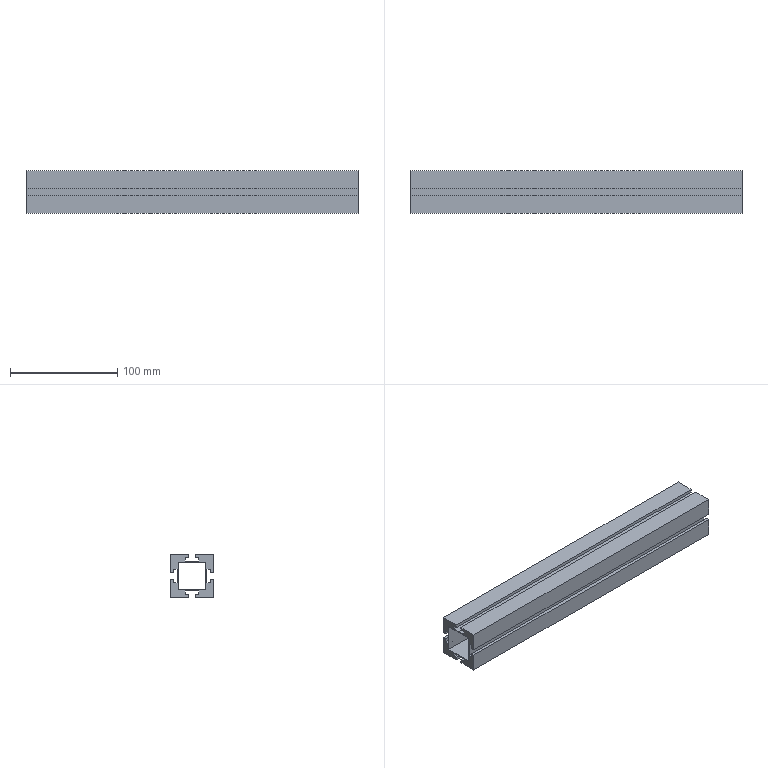Part | SolidWorks | features Extrusion 1 | 1 solid | 42 faces | box 310 x 40 x 40 mm | volume 215760 mm3 | plane 42
STEP:
#1=CARTESIAN_POINT('',(310.,3.,-20.));
#2=VERTEX_POINT('',#1);
#3=CARTESIAN_POINT('',(310.,20.,-20.));
#4=VERTEX_POINT('',#3);
#5=CARTESIAN_POINT('',(310.,3.,-20.));
#6=DIRECTION('',(0.,1.,0.));
#7=VECTOR('',#6,1000.);
#8=LINE('',#5,#7);
#9=EDGE_CURVE('',#2,#4,#8,.T.);
#10=ORIENTED_EDGE('',*,*,#9,.T.);
#11=CARTESIAN_POINT('',(310.,20.,-3.));
#12=VERTEX_POINT('',#11);
#13=CARTESIAN_POINT('',(310.,20.,-3.));
#14=DIRECTION('',(0.,0.,1.));
#15=VECTOR('',#14,1000.);
#16=LINE('',#13,#15);
#17=EDGE_CURVE('',#4,#12,#16,.T.);
#18=ORIENTED_EDGE('',*,*,#17,.T.);
#19=CARTESIAN_POINT('',(310.,17.,-3.));
#20=VERTEX_POINT('',#19);
#21=CARTESIAN_POINT('',(310.,20.,-3.));
#22=DIRECTION('',(0.,-1.,0.));
#23=VECTOR('',#22,1000.);
#24=LINE('',#21,#23);
#25=EDGE_CURVE('',#12,#20,#24,.T.);
#26=ORIENTED_EDGE('',*,*,#25,.T.);
#27=CARTESIAN_POINT('',(310.,17.,-6.5));
#28=VERTEX_POINT('',#27);
#29=CARTESIAN_POINT('',(310.,17.,-3.));
#30=DIRECTION('',(0.,0.,-1.));
#31=VECTOR('',#30,1000.);
#32=LINE('',#29,#31);
#33=EDGE_CURVE('',#20,#28,#32,.T.);
#34=ORIENTED_EDGE('',*,*,#33,.T.);
#35=CARTESIAN_POINT('',(310.,14.,-6.5));
#36=VERTEX_POINT('',#35);
#37=CARTESIAN_POINT('',(310.,17.,-6.5));
#38=DIRECTION('',(0.,-1.,0.));
#39=VECTOR('',#38,1000.);
#40=LINE('',#37,#39);
#41=EDGE_CURVE('',#28,#36,#40,.T.);
#42=ORIENTED_EDGE('',*,*,#41,.T.);
#43=CARTESIAN_POINT('',(310.,14.,6.5));
#44=VERTEX_POINT('',#43);
#45=CARTESIAN_POINT('',(310.,14.,6.5));
#46=DIRECTION('',(0.,0.,1.));
#47=VECTOR('',#46,1000.);
#48=LINE('',#45,#47);
#49=EDGE_CURVE('',#36,#44,#48,.T.);
#50=ORIENTED_EDGE('',*,*,#49,.T.);
#51=CARTESIAN_POINT('',(310.,17.,6.5));
#52=VERTEX_POINT('',#51);
#53=CARTESIAN_POINT('',(310.,17.,6.5));
#54=DIRECTION('',(0.,1.,0.));
#55=VECTOR('',#54,1000.);
#56=LINE('',#53,#55);
#57=EDGE_CURVE('',#44,#52,#56,.T.);
#58=ORIENTED_EDGE('',*,*,#57,.T.);
#59=CARTESIAN_POINT('',(310.,17.,3.));
#60=VERTEX_POINT('',#59);
#61=CARTESIAN_POINT('',(310.,17.,6.5));
#62=DIRECTION('',(0.,0.,-1.));
#63=VECTOR('',#62,1000.);
#64=LINE('',#61,#63);
#65=EDGE_CURVE('',#52,#60,#64,.T.);
#66=ORIENTED_EDGE('',*,*,#65,.T.);
#67=CARTESIAN_POINT('',(310.,20.,3.));
#68=VERTEX_POINT('',#67);
#69=CARTESIAN_POINT('',(310.,20.,3.));
#70=DIRECTION('',(0.,1.,0.));
#71=VECTOR('',#70,1000.);
#72=LINE('',#69,#71);
#73=EDGE_CURVE('',#60,#68,#72,.T.);
#74=ORIENTED_EDGE('',*,*,#73,.T.);
#75=CARTESIAN_POINT('',(310.,20.,20.));
#76=VERTEX_POINT('',#75);
#77=CARTESIAN_POINT('',(310.,20.,20.));
#78=DIRECTION('',(0.,0.,1.));
#79=VECTOR('',#78,1000.);
#80=LINE('',#77,#79);
#81=EDGE_CURVE('',#68,#76,#80,.T.);
#82=ORIENTED_EDGE('',*,*,#81,.T.);
#83=CARTESIAN_POINT('',(310.,3.,20.));
#84=VERTEX_POINT('',#83);
#85=CARTESIAN_POINT('',(310.,3.,20.));
#86=DIRECTION('',(0.,-1.,0.));
#87=VECTOR('',#86,1000.);
#88=LINE('',#85,#87);
#89=EDGE_CURVE('',#76,#84,#88,.T.);
#90=ORIENTED_EDGE('',*,*,#89,.T.);
#91=CARTESIAN_POINT('',(310.,3.,17.));
#92=VERTEX_POINT('',#91);
#93=CARTESIAN_POINT('',(310.,3.,17.));
#94=DIRECTION('',(0.,0.,-1.));
#95=VECTOR('',#94,1000.);
#96=LINE('',#93,#95);
#97=EDGE_CURVE('',#84,#92,#96,.T.);
#98=ORIENTED_EDGE('',*,*,#97,.T.);
#99=CARTESIAN_POINT('',(310.,6.5,17.));
#100=VERTEX_POINT('',#99);
#101=CARTESIAN_POINT('',(310.,3.,17.));
#102=DIRECTION('',(0.,1.,0.));
#103=VECTOR('',#102,1000.);
#104=LINE('',#101,#103);
#105=EDGE_CURVE('',#92,#100,#104,.T.);
#106=ORIENTED_EDGE('',*,*,#105,.T.);
#107=CARTESIAN_POINT('',(310.,6.5,14.));
#108=VERTEX_POINT('',#107);
#109=CARTESIAN_POINT('',(310.,6.5,14.));
#110=DIRECTION('',(0.,0.,-1.));
#111=VECTOR('',#110,1000.);
#112=LINE('',#109,#111);
#113=EDGE_CURVE('',#100,#108,#112,.T.);
#114=ORIENTED_EDGE('',*,*,#113,.T.);
#115=CARTESIAN_POINT('',(310.,-6.5,14.));
#116=VERTEX_POINT('',#115);
#117=CARTESIAN_POINT('',(310.,-6.5,14.));
#118=DIRECTION('',(0.,-1.,0.));
#119=VECTOR('',#118,1000.);
#120=LINE('',#117,#119);
#121=EDGE_CURVE('',#108,#116,#120,.T.);
#122=ORIENTED_EDGE('',*,*,#121,.T.);
#123=CARTESIAN_POINT('',(310.,-6.5,17.));
#124=VERTEX_POINT('',#123);
#125=CARTESIAN_POINT('',(310.,-6.5,14.));
#126=DIRECTION('',(0.,0.,1.));
#127=VECTOR('',#126,1000.);
#128=LINE('',#125,#127);
#129=EDGE_CURVE('',#116,#124,#128,.T.);
#130=ORIENTED_EDGE('',*,*,#129,.T.);
#131=CARTESIAN_POINT('',(310.,-3.,17.));
#132=VERTEX_POINT('',#131);
#133=CARTESIAN_POINT('',(310.,-6.5,17.));
#134=DIRECTION('',(0.,1.,0.));
#135=VECTOR('',#134,1000.);
#136=LINE('',#133,#135);
#137=EDGE_CURVE('',#124,#132,#136,.T.);
#138=ORIENTED_EDGE('',*,*,#137,.T.);
#139=CARTESIAN_POINT('',(310.,-3.,20.));
#140=VERTEX_POINT('',#139);
#141=CARTESIAN_POINT('',(310.,-3.,17.));
#142=DIRECTION('',(0.,0.,1.));
#143=VECTOR('',#142,1000.);
#144=LINE('',#141,#143);
#145=EDGE_CURVE('',#132,#140,#144,.T.);
#146=ORIENTED_EDGE('',*,*,#145,.T.);
#147=CARTESIAN_POINT('',(310.,-20.,20.));
#148=VERTEX_POINT('',#147);
#149=CARTESIAN_POINT('',(310.,-20.,20.));
#150=DIRECTION('',(0.,-1.,0.));
#151=VECTOR('',#150,1000.);
#152=LINE('',#149,#151);
#153=EDGE_CURVE('',#140,#148,#152,.T.);
#154=ORIENTED_EDGE('',*,*,#153,.T.);
#155=CARTESIAN_POINT('',(310.,-20.,3.));
#156=VERTEX_POINT('',#155);
#157=CARTESIAN_POINT('',(310.,-20.,20.));
#158=DIRECTION('',(0.,0.,-1.));
#159=VECTOR('',#158,1000.);
#160=LINE('',#157,#159);
#161=EDGE_CURVE('',#148,#156,#160,.T.);
#162=ORIENTED_EDGE('',*,*,#161,.T.);
#163=CARTESIAN_POINT('',(310.,-17.,3.));
#164=VERTEX_POINT('',#163);
#165=CARTESIAN_POINT('',(310.,-20.,3.));
#166=DIRECTION('',(0.,1.,0.));
#167=VECTOR('',#166,1000.);
#168=LINE('',#165,#167);
#169=EDGE_CURVE('',#156,#164,#168,.T.);
#170=ORIENTED_EDGE('',*,*,#169,.T.);
#171=CARTESIAN_POINT('',(310.,-17.,6.5));
#172=VERTEX_POINT('',#171);
#173=CARTESIAN_POINT('',(310.,-17.,6.5));
#174=DIRECTION('',(0.,0.,1.));
#175=VECTOR('',#174,1000.);
#176=LINE('',#173,#175);
#177=EDGE_CURVE('',#164,#172,#176,.T.);
#178=ORIENTED_EDGE('',*,*,#177,.T.);
#179=CARTESIAN_POINT('',(310.,-14.,6.5));
#180=VERTEX_POINT('',#179);
#181=CARTESIAN_POINT('',(310.,-17.,6.5));
#182=DIRECTION('',(0.,1.,0.));
#183=VECTOR('',#182,1000.);
#184=LINE('',#181,#183);
#185=EDGE_CURVE('',#172,#180,#184,.T.);
#186=ORIENTED_EDGE('',*,*,#185,.T.);
#187=CARTESIAN_POINT('',(310.,-14.,-6.5));
#188=VERTEX_POINT('',#187);
#189=CARTESIAN_POINT('',(310.,-14.,6.5));
#190=DIRECTION('',(0.,0.,-1.));
#191=VECTOR('',#190,1000.);
#192=LINE('',#189,#191);
#193=EDGE_CURVE('',#180,#188,#192,.T.);
#194=ORIENTED_EDGE('',*,*,#193,.T.);
#195=CARTESIAN_POINT('',(310.,-17.,-6.5));
#196=VERTEX_POINT('',#195);
#197=CARTESIAN_POINT('',(310.,-17.,-6.5));
#198=DIRECTION('',(0.,-1.,0.));
#199=VECTOR('',#198,1000.);
#200=LINE('',#197,#199);
#201=EDGE_CURVE('',#188,#196,#200,.T.);
#202=ORIENTED_EDGE('',*,*,#201,.T.);
#203=CARTESIAN_POINT('',(310.,-17.,-3.));
#204=VERTEX_POINT('',#203);
#205=CARTESIAN_POINT('',(310.,-17.,-3.));
#206=DIRECTION('',(0.,0.,1.));
#207=VECTOR('',#206,1000.);
#208=LINE('',#205,#207);
#209=EDGE_CURVE('',#196,#204,#208,.T.);
#210=ORIENTED_EDGE('',*,*,#209,.T.);
#211=CARTESIAN_POINT('',(310.,-20.,-3.));
#212=VERTEX_POINT('',#211);
#213=CARTESIAN_POINT('',(310.,-20.,-3.));
#214=DIRECTION('',(0.,-1.,0.));
#215=VECTOR('',#214,1000.);
#216=LINE('',#213,#215);
#217=EDGE_CURVE('',#204,#212,#216,.T.);
#218=ORIENTED_EDGE('',*,*,#217,.T.);
#219=CARTESIAN_POINT('',(310.,-20.,-20.));
#220=VERTEX_POINT('',#219);
#221=CARTESIAN_POINT('',(310.,-20.,-3.));
#222=DIRECTION('',(0.,0.,-1.));
#223=VECTOR('',#222,1000.);
#224=LINE('',#221,#223);
#225=EDGE_CURVE('',#212,#220,#224,.T.);
#226=ORIENTED_EDGE('',*,*,#225,.T.);
#227=CARTESIAN_POINT('',(310.,-3.,-20.));
#228=VERTEX_POINT('',#227);
#229=CARTESIAN_POINT('',(310.,-20.,-20.));
#230=DIRECTION('',(0.,1.,0.));
#231=VECTOR('',#230,1000.);
#232=LINE('',#229,#231);
#233=EDGE_CURVE('',#220,#228,#232,.T.);
#234=ORIENTED_EDGE('',*,*,#233,.T.);
#235=CARTESIAN_POINT('',(310.,-3.,-17.));
#236=VERTEX_POINT('',#235);
#237=CARTESIAN_POINT('',(310.,-3.,-17.));
#238=DIRECTION('',(0.,0.,1.));
#239=VECTOR('',#238,1000.);
#240=LINE('',#237,#239);
#241=EDGE_CURVE('',#228,#236,#240,.T.);
#242=ORIENTED_EDGE('',*,*,#241,.T.);
#243=CARTESIAN_POINT('',(310.,-6.5,-17.));
#244=VERTEX_POINT('',#243);
#245=CARTESIAN_POINT('',(310.,-6.5,-17.));
#246=DIRECTION('',(0.,-1.,0.));
#247=VECTOR('',#246,1000.);
#248=LINE('',#245,#247);
#249=EDGE_CURVE('',#236,#244,#248,.T.);
#250=ORIENTED_EDGE('',*,*,#249,.T.);
#251=CARTESIAN_POINT('',(310.,-6.5,-14.));
#252=VERTEX_POINT('',#251);
#253=CARTESIAN_POINT('',(310.,-6.5,-14.));
#254=DIRECTION('',(0.,0.,1.));
#255=VECTOR('',#254,1000.);
#256=LINE('',#253,#255);
#257=EDGE_CURVE('',#244,#252,#256,.T.);
#258=ORIENTED_EDGE('',*,*,#257,.T.);
#259=CARTESIAN_POINT('',(310.,6.5,-14.));
#260=VERTEX_POINT('',#259);
#261=CARTESIAN_POINT('',(310.,-6.5,-14.));
#262=DIRECTION('',(0.,1.,0.));
#263=VECTOR('',#262,1000.);
#264=LINE('',#261,#263);
#265=EDGE_CURVE('',#252,#260,#264,.T.);
#266=ORIENTED_EDGE('',*,*,#265,.T.);
#267=CARTESIAN_POINT('',(310.,6.5,-17.));
#268=VERTEX_POINT('',#267);
#269=CARTESIAN_POINT('',(310.,6.5,-14.));
#270=DIRECTION('',(0.,0.,-1.));
#271=VECTOR('',#270,1000.);
#272=LINE('',#269,#271);
#273=EDGE_CURVE('',#260,#268,#272,.T.);
#274=ORIENTED_EDGE('',*,*,#273,.T.);
#275=CARTESIAN_POINT('',(310.,3.,-17.));
#276=VERTEX_POINT('',#275);
#277=CARTESIAN_POINT('',(310.,3.,-17.));
#278=DIRECTION('',(0.,-1.,0.));
#279=VECTOR('',#278,1000.);
#280=LINE('',#277,#279);
#281=EDGE_CURVE('',#268,#276,#280,.T.);
#282=ORIENTED_EDGE('',*,*,#281,.T.);
#283=CARTESIAN_POINT('',(310.,3.,-17.));
#284=DIRECTION('',(0.,0.,-1.));
#285=VECTOR('',#284,1000.);
#286=LINE('',#283,#285);
#287=EDGE_CURVE('',#276,#2,#286,.T.);
#288=ORIENTED_EDGE('',*,*,#287,.T.);
#289=EDGE_LOOP('',(#10,#18,#26,#34,#42,#50,#58,#66,#74,#82,#90,#98,#106,#114,#122,#130,#138,#146,#154,#162,#170,#178,#186,#194,#202,#210,#218,#226,#234,#242,#250,#258,#266,#274,#282,#288));
#290=FACE_OUTER_BOUND('',#289,.T.);
#291=CARTESIAN_POINT('',(310.,-13.,-13.));
#292=VERTEX_POINT('',#291);
#293=CARTESIAN_POINT('',(310.,13.,-13.));
#294=VERTEX_POINT('',#293);
#295=CARTESIAN_POINT('',(310.,-13.,-13.));
#296=DIRECTION('',(0.,1.,0.));
#297=VECTOR('',#296,1000.);
#298=LINE('',#295,#297);
#299=EDGE_CURVE('',#292,#294,#298,.T.);
#300=ORIENTED_EDGE('',*,*,#299,.F.);
#301=CARTESIAN_POINT('',(310.,-13.,13.));
#302=VERTEX_POINT('',#301);
#303=CARTESIAN_POINT('',(310.,-13.,13.));
#304=DIRECTION('',(0.,0.,-1.));
#305=VECTOR('',#304,1000.);
#306=LINE('',#303,#305);
#307=EDGE_CURVE('',#302,#292,#306,.T.);
#308=ORIENTED_EDGE('',*,*,#307,.F.);
#309=CARTESIAN_POINT('',(310.,13.,13.));
#310=VERTEX_POINT('',#309);
#311=CARTESIAN_POINT('',(310.,-13.,13.));
#312=DIRECTION('',(0.,-1.,0.));
#313=VECTOR('',#312,1000.);
#314=LINE('',#311,#313);
#315=EDGE_CURVE('',#310,#302,#314,.T.);
#316=ORIENTED_EDGE('',*,*,#315,.F.);
#317=CARTESIAN_POINT('',(310.,13.,13.));
#318=DIRECTION('',(0.,0.,1.));
#319=VECTOR('',#318,1000.);
#320=LINE('',#317,#319);
#321=EDGE_CURVE('',#294,#310,#320,.T.);
#322=ORIENTED_EDGE('',*,*,#321,.F.);
#323=EDGE_LOOP('',(#300,#308,#316,#322));
#324=FACE_BOUND('',#323,.T.);
#325=CARTESIAN_POINT('',(310.,20.,-20.));
#326=DIRECTION('',(-1.,0.,0.));
#327=DIRECTION('',(0.,0.,1.));
#328=AXIS2_PLACEMENT_3D('',#325,#326,#327);
#329=PLANE('',#328);
#330=ADVANCED_FACE('',(#290,#324),#329,.F.);
#331=CARTESIAN_POINT('',(0.,3.,-20.));
#332=VERTEX_POINT('',#331);
#333=CARTESIAN_POINT('',(0.,20.,-20.));
#334=VERTEX_POINT('',#333);
#335=CARTESIAN_POINT('',(0.,3.,-20.));
#336=DIRECTION('',(0.,1.,0.));
#337=VECTOR('',#336,1000.);
#338=LINE('',#335,#337);
#339=EDGE_CURVE('',#332,#334,#338,.T.);
#340=ORIENTED_EDGE('',*,*,#339,.F.);
#341=CARTESIAN_POINT('',(0.,3.,-17.));
#342=VERTEX_POINT('',#341);
#343=CARTESIAN_POINT('',(0.,3.,-17.));
#344=DIRECTION('',(0.,0.,-1.));
#345=VECTOR('',#344,1000.);
#346=LINE('',#343,#345);
#347=EDGE_CURVE('',#342,#332,#346,.T.);
#348=ORIENTED_EDGE('',*,*,#347,.F.);
#349=CARTESIAN_POINT('',(0.,6.5,-17.));
#350=VERTEX_POINT('',#349);
#351=CARTESIAN_POINT('',(0.,3.,-17.));
#352=DIRECTION('',(0.,-1.,0.));
#353=VECTOR('',#352,1000.);
#354=LINE('',#351,#353);
#355=EDGE_CURVE('',#350,#342,#354,.T.);
#356=ORIENTED_EDGE('',*,*,#355,.F.);
#357=CARTESIAN_POINT('',(0.,6.5,-14.));
#358=VERTEX_POINT('',#357);
#359=CARTESIAN_POINT('',(0.,6.5,-14.));
#360=DIRECTION('',(0.,0.,-1.));
#361=VECTOR('',#360,1000.);
#362=LINE('',#359,#361);
#363=EDGE_CURVE('',#358,#350,#362,.T.);
#364=ORIENTED_EDGE('',*,*,#363,.F.);
#365=CARTESIAN_POINT('',(0.,-6.5,-14.));
#366=VERTEX_POINT('',#365);
#367=CARTESIAN_POINT('',(0.,-6.5,-14.));
#368=DIRECTION('',(0.,1.,0.));
#369=VECTOR('',#368,1000.);
#370=LINE('',#367,#369);
#371=EDGE_CURVE('',#366,#358,#370,.T.);
#372=ORIENTED_EDGE('',*,*,#371,.F.);
#373=CARTESIAN_POINT('',(0.,-6.5,-17.));
#374=VERTEX_POINT('',#373);
#375=CARTESIAN_POINT('',(0.,-6.5,-14.));
#376=DIRECTION('',(0.,0.,1.));
#377=VECTOR('',#376,1000.);
#378=LINE('',#375,#377);
#379=EDGE_CURVE('',#374,#366,#378,.T.);
#380=ORIENTED_EDGE('',*,*,#379,.F.);
#381=CARTESIAN_POINT('',(0.,-3.,-17.));
#382=VERTEX_POINT('',#381);
#383=CARTESIAN_POINT('',(0.,-6.5,-17.));
#384=DIRECTION('',(0.,-1.,0.));
#385=VECTOR('',#384,1000.);
#386=LINE('',#383,#385);
#387=EDGE_CURVE('',#382,#374,#386,.T.);
#388=ORIENTED_EDGE('',*,*,#387,.F.);
#389=CARTESIAN_POINT('',(0.,-3.,-20.));
#390=VERTEX_POINT('',#389);
#391=CARTESIAN_POINT('',(0.,-3.,-17.));
#392=DIRECTION('',(0.,0.,1.));
#393=VECTOR('',#392,1000.);
#394=LINE('',#391,#393);
#395=EDGE_CURVE('',#390,#382,#394,.T.);
#396=ORIENTED_EDGE('',*,*,#395,.F.);
#397=CARTESIAN_POINT('',(0.,-20.,-20.));
#398=VERTEX_POINT('',#397);
#399=CARTESIAN_POINT('',(0.,-20.,-20.));
#400=DIRECTION('',(0.,1.,0.));
#401=VECTOR('',#400,1000.);
#402=LINE('',#399,#401);
#403=EDGE_CURVE('',#398,#390,#402,.T.);
#404=ORIENTED_EDGE('',*,*,#403,.F.);
#405=CARTESIAN_POINT('',(0.,-20.,-3.));
#406=VERTEX_POINT('',#405);
#407=CARTESIAN_POINT('',(0.,-20.,-3.));
#408=DIRECTION('',(0.,0.,-1.));
#409=VECTOR('',#408,1000.);
#410=LINE('',#407,#409);
#411=EDGE_CURVE('',#406,#398,#410,.T.);
#412=ORIENTED_EDGE('',*,*,#411,.F.);
#413=CARTESIAN_POINT('',(0.,-17.,-3.));
#414=VERTEX_POINT('',#413);
#415=CARTESIAN_POINT('',(0.,-20.,-3.));
#416=DIRECTION('',(0.,-1.,0.));
#417=VECTOR('',#416,1000.);
#418=LINE('',#415,#417);
#419=EDGE_CURVE('',#414,#406,#418,.T.);
#420=ORIENTED_EDGE('',*,*,#419,.F.);
#421=CARTESIAN_POINT('',(0.,-17.,-6.5));
#422=VERTEX_POINT('',#421);
#423=CARTESIAN_POINT('',(0.,-17.,-3.));
#424=DIRECTION('',(0.,0.,1.));
#425=VECTOR('',#424,1000.);
#426=LINE('',#423,#425);
#427=EDGE_CURVE('',#422,#414,#426,.T.);
#428=ORIENTED_EDGE('',*,*,#427,.F.);
#429=CARTESIAN_POINT('',(0.,-14.,-6.5));
#430=VERTEX_POINT('',#429);
#431=CARTESIAN_POINT('',(0.,-17.,-6.5));
#432=DIRECTION('',(0.,-1.,0.));
#433=VECTOR('',#432,1000.);
#434=LINE('',#431,#433);
#435=EDGE_CURVE('',#430,#422,#434,.T.);
#436=ORIENTED_EDGE('',*,*,#435,.F.);
#437=CARTESIAN_POINT('',(0.,-14.,6.5));
#438=VERTEX_POINT('',#437);
#439=CARTESIAN_POINT('',(0.,-14.,6.5));
#440=DIRECTION('',(0.,0.,-1.));
#441=VECTOR('',#440,1000.);
#442=LINE('',#439,#441);
#443=EDGE_CURVE('',#438,#430,#442,.T.);
#444=ORIENTED_EDGE('',*,*,#443,.F.);
#445=CARTESIAN_POINT('',(0.,-17.,6.5));
#446=VERTEX_POINT('',#445);
#447=CARTESIAN_POINT('',(0.,-17.,6.5));
#448=DIRECTION('',(0.,1.,0.));
#449=VECTOR('',#448,1000.);
#450=LINE('',#447,#449);
#451=EDGE_CURVE('',#446,#438,#450,.T.);
#452=ORIENTED_EDGE('',*,*,#451,.F.);
#453=CARTESIAN_POINT('',(0.,-17.,3.));
#454=VERTEX_POINT('',#453);
#455=CARTESIAN_POINT('',(0.,-17.,6.5));
#456=DIRECTION('',(0.,0.,1.));
#457=VECTOR('',#456,1000.);
#458=LINE('',#455,#457);
#459=EDGE_CURVE('',#454,#446,#458,.T.);
#460=ORIENTED_EDGE('',*,*,#459,.F.);
#461=CARTESIAN_POINT('',(0.,-20.,3.));
#462=VERTEX_POINT('',#461);
#463=CARTESIAN_POINT('',(0.,-20.,3.));
#464=DIRECTION('',(0.,1.,0.));
#465=VECTOR('',#464,1000.);
#466=LINE('',#463,#465);
#467=EDGE_CURVE('',#462,#454,#466,.T.);
#468=ORIENTED_EDGE('',*,*,#467,.F.);
#469=CARTESIAN_POINT('',(0.,-20.,20.));
#470=VERTEX_POINT('',#469);
#471=CARTESIAN_POINT('',(0.,-20.,20.));
#472=DIRECTION('',(0.,0.,-1.));
#473=VECTOR('',#472,1000.);
#474=LINE('',#471,#473);
#475=EDGE_CURVE('',#470,#462,#474,.T.);
#476=ORIENTED_EDGE('',*,*,#475,.F.);
#477=CARTESIAN_POINT('',(0.,-3.,20.));
#478=VERTEX_POINT('',#477);
#479=CARTESIAN_POINT('',(0.,-20.,20.));
#480=DIRECTION('',(0.,-1.,0.));
#481=VECTOR('',#480,1000.);
#482=LINE('',#479,#481);
#483=EDGE_CURVE('',#478,#470,#482,.T.);
#484=ORIENTED_EDGE('',*,*,#483,.F.);
#485=CARTESIAN_POINT('',(0.,-3.,17.));
#486=VERTEX_POINT('',#485);
#487=CARTESIAN_POINT('',(0.,-3.,17.));
#488=DIRECTION('',(0.,0.,1.));
#489=VECTOR('',#488,1000.);
#490=LINE('',#487,#489);
#491=EDGE_CURVE('',#486,#478,#490,.T.);
#492=ORIENTED_EDGE('',*,*,#491,.F.);
#493=CARTESIAN_POINT('',(0.,-6.5,17.));
#494=VERTEX_POINT('',#493);
#495=CARTESIAN_POINT('',(0.,-6.5,17.));
#496=DIRECTION('',(0.,1.,0.));
#497=VECTOR('',#496,1000.);
#498=LINE('',#495,#497);
#499=EDGE_CURVE('',#494,#486,#498,.T.);
#500=ORIENTED_EDGE('',*,*,#499,.F.);
#501=CARTESIAN_POINT('',(0.,-6.5,14.));
#502=VERTEX_POINT('',#501);
#503=CARTESIAN_POINT('',(0.,-6.5,14.));
#504=DIRECTION('',(0.,0.,1.));
#505=VECTOR('',#504,1000.);
#506=LINE('',#503,#505);
#507=EDGE_CURVE('',#502,#494,#506,.T.);
#508=ORIENTED_EDGE('',*,*,#507,.F.);
#509=CARTESIAN_POINT('',(0.,6.5,14.));
#510=VERTEX_POINT('',#509);
#511=CARTESIAN_POINT('',(0.,-6.5,14.));
#512=DIRECTION('',(0.,-1.,0.));
#513=VECTOR('',#512,1000.);
#514=LINE('',#511,#513);
#515=EDGE_CURVE('',#510,#502,#514,.T.);
#516=ORIENTED_EDGE('',*,*,#515,.F.);
#517=CARTESIAN_POINT('',(0.,6.5,17.));
#518=VERTEX_POINT('',#517);
#519=CARTESIAN_POINT('',(0.,6.5,14.));
#520=DIRECTION('',(0.,0.,-1.));
#521=VECTOR('',#520,1000.);
#522=LINE('',#519,#521);
#523=EDGE_CURVE('',#518,#510,#522,.T.);
#524=ORIENTED_EDGE('',*,*,#523,.F.);
#525=CARTESIAN_POINT('',(0.,3.,17.));
#526=VERTEX_POINT('',#525);
#527=CARTESIAN_POINT('',(0.,3.,17.));
#528=DIRECTION('',(0.,1.,0.));
#529=VECTOR('',#528,1000.);
#530=LINE('',#527,#529);
#531=EDGE_CURVE('',#526,#518,#530,.T.);
#532=ORIENTED_EDGE('',*,*,#531,.F.);
#533=CARTESIAN_POINT('',(0.,3.,20.));
#534=VERTEX_POINT('',#533);
#535=CARTESIAN_POINT('',(0.,3.,17.));
#536=DIRECTION('',(0.,0.,-1.));
#537=VECTOR('',#536,1000.);
#538=LINE('',#535,#537);
#539=EDGE_CURVE('',#534,#526,#538,.T.);
#540=ORIENTED_EDGE('',*,*,#539,.F.);
#541=CARTESIAN_POINT('',(0.,20.,20.));
#542=VERTEX_POINT('',#541);
#543=CARTESIAN_POINT('',(0.,3.,20.));
#544=DIRECTION('',(0.,-1.,0.));
#545=VECTOR('',#544,1000.);
#546=LINE('',#543,#545);
#547=EDGE_CURVE('',#542,#534,#546,.T.);
#548=ORIENTED_EDGE('',*,*,#547,.F.);
#549=CARTESIAN_POINT('',(0.,20.,3.));
#550=VERTEX_POINT('',#549);
#551=CARTESIAN_POINT('',(0.,20.,20.));
#552=DIRECTION('',(0.,0.,1.));
#553=VECTOR('',#552,1000.);
#554=LINE('',#551,#553);
#555=EDGE_CURVE('',#550,#542,#554,.T.);
#556=ORIENTED_EDGE('',*,*,#555,.F.);
#557=CARTESIAN_POINT('',(0.,17.,3.));
#558=VERTEX_POINT('',#557);
#559=CARTESIAN_POINT('',(0.,20.,3.));
#560=DIRECTION('',(0.,1.,0.));
#561=VECTOR('',#560,1000.);
#562=LINE('',#559,#561);
#563=EDGE_CURVE('',#558,#550,#562,.T.);
#564=ORIENTED_EDGE('',*,*,#563,.F.);
#565=CARTESIAN_POINT('',(0.,17.,6.5));
#566=VERTEX_POINT('',#565);
#567=CARTESIAN_POINT('',(0.,17.,6.5));
#568=DIRECTION('',(0.,0.,-1.));
#569=VECTOR('',#568,1000.);
#570=LINE('',#567,#569);
#571=EDGE_CURVE('',#566,#558,#570,.T.);
#572=ORIENTED_EDGE('',*,*,#571,.F.);
#573=CARTESIAN_POINT('',(0.,14.,6.5));
#574=VERTEX_POINT('',#573);
#575=CARTESIAN_POINT('',(0.,17.,6.5));
#576=DIRECTION('',(0.,1.,0.));
#577=VECTOR('',#576,1000.);
#578=LINE('',#575,#577);
#579=EDGE_CURVE('',#574,#566,#578,.T.);
#580=ORIENTED_EDGE('',*,*,#579,.F.);
#581=CARTESIAN_POINT('',(0.,14.,-6.5));
#582=VERTEX_POINT('',#581);
#583=CARTESIAN_POINT('',(0.,14.,6.5));
#584=DIRECTION('',(0.,0.,1.));
#585=VECTOR('',#584,1000.);
#586=LINE('',#583,#585);
#587=EDGE_CURVE('',#582,#574,#586,.T.);
#588=ORIENTED_EDGE('',*,*,#587,.F.);
#589=CARTESIAN_POINT('',(0.,17.,-6.5));
#590=VERTEX_POINT('',#589);
#591=CARTESIAN_POINT('',(0.,17.,-6.5));
#592=DIRECTION('',(0.,-1.,0.));
#593=VECTOR('',#592,1000.);
#594=LINE('',#591,#593);
#595=EDGE_CURVE('',#590,#582,#594,.T.);
#596=ORIENTED_EDGE('',*,*,#595,.F.);
#597=CARTESIAN_POINT('',(0.,17.,-3.));
#598=VERTEX_POINT('',#597);
#599=CARTESIAN_POINT('',(0.,17.,-3.));
#600=DIRECTION('',(0.,0.,-1.));
#601=VECTOR('',#600,1000.);
#602=LINE('',#599,#601);
#603=EDGE_CURVE('',#598,#590,#602,.T.);
#604=ORIENTED_EDGE('',*,*,#603,.F.);
#605=CARTESIAN_POINT('',(0.,20.,-3.));
#606=VERTEX_POINT('',#605);
#607=CARTESIAN_POINT('',(0.,20.,-3.));
#608=DIRECTION('',(0.,-1.,0.));
#609=VECTOR('',#608,1000.);
#610=LINE('',#607,#609);
#611=EDGE_CURVE('',#606,#598,#610,.T.);
#612=ORIENTED_EDGE('',*,*,#611,.F.);
#613=CARTESIAN_POINT('',(0.,20.,-3.));
#614=DIRECTION('',(0.,0.,1.));
#615=VECTOR('',#614,1000.);
#616=LINE('',#613,#615);
#617=EDGE_CURVE('',#334,#606,#616,.T.);
#618=ORIENTED_EDGE('',*,*,#617,.F.);
#619=EDGE_LOOP('',(#340,#348,#356,#364,#372,#380,#388,#396,#404,#412,#420,#428,#436,#444,#452,#460,#468,#476,#484,#492,#500,#508,#516,#524,#532,#540,#548,#556,#564,#572,#580,#588,#596,#604,#612,#618));
#620=FACE_OUTER_BOUND('',#619,.T.);
#621=CARTESIAN_POINT('',(0.,-13.,13.));
#622=VERTEX_POINT('',#621);
#623=CARTESIAN_POINT('',(0.,-13.,-13.));
#624=VERTEX_POINT('',#623);
#625=CARTESIAN_POINT('',(0.,-13.,13.));
#626=DIRECTION('',(0.,0.,-1.));
#627=VECTOR('',#626,1000.);
#628=LINE('',#625,#627);
#629=EDGE_CURVE('',#622,#624,#628,.T.);
#630=ORIENTED_EDGE('',*,*,#629,.T.);
#631=CARTESIAN_POINT('',(0.,13.,-13.));
#632=VERTEX_POINT('',#631);
#633=CARTESIAN_POINT('',(0.,-13.,-13.));
#634=DIRECTION('',(0.,1.,0.));
#635=VECTOR('',#634,1000.);
#636=LINE('',#633,#635);
#637=EDGE_CURVE('',#624,#632,#636,.T.);
#638=ORIENTED_EDGE('',*,*,#637,.T.);
#639=CARTESIAN_POINT('',(0.,13.,13.));
#640=VERTEX_POINT('',#639);
#641=CARTESIAN_POINT('',(0.,13.,13.));
#642=DIRECTION('',(0.,0.,1.));
#643=VECTOR('',#642,1000.);
#644=LINE('',#641,#643);
#645=EDGE_CURVE('',#632,#640,#644,.T.);
#646=ORIENTED_EDGE('',*,*,#645,.T.);
#647=CARTESIAN_POINT('',(0.,-13.,13.));
#648=DIRECTION('',(0.,-1.,0.));
#649=VECTOR('',#648,1000.);
#650=LINE('',#647,#649);
#651=EDGE_CURVE('',#640,#622,#650,.T.);
#652=ORIENTED_EDGE('',*,*,#651,.T.);
#653=EDGE_LOOP('',(#630,#638,#646,#652));
#654=FACE_BOUND('',#653,.T.);
#655=CARTESIAN_POINT('',(0.,20.,-20.));
#656=DIRECTION('',(-1.,0.,0.));
#657=DIRECTION('',(0.,0.,1.));
#658=AXIS2_PLACEMENT_3D('',#655,#656,#657);
#659=PLANE('',#658);
#660=ADVANCED_FACE('',(#620,#654),#659,.T.);
#661=ORIENTED_EDGE('',*,*,#339,.T.);
#662=CARTESIAN_POINT('',(310.,20.,-20.));
#663=DIRECTION('',(-1.,0.,0.));
#664=VECTOR('',#663,1000.);
#665=LINE('',#662,#664);
#666=EDGE_CURVE('',#4,#334,#665,.T.);
#667=ORIENTED_EDGE('',*,*,#666,.F.);
#668=ORIENTED_EDGE('',*,*,#9,.F.);
#669=CARTESIAN_POINT('',(310.,3.,-20.));
#670=DIRECTION('',(-1.,0.,0.));
#671=VECTOR('',#670,1000.);
#672=LINE('',#669,#671);
#673=EDGE_CURVE('',#2,#332,#672,.T.);
#674=ORIENTED_EDGE('',*,*,#673,.T.);
#675=EDGE_LOOP('',(#661,#667,#668,#674));
#676=FACE_OUTER_BOUND('',#675,.T.);
#677=CARTESIAN_POINT('',(310.,3.,-20.));
#678=DIRECTION('',(0.,0.,1.));
#679=DIRECTION('',(0.,-1.,0.));
#680=AXIS2_PLACEMENT_3D('',#677,#678,#679);
#681=PLANE('',#680);
#682=ADVANCED_FACE('',(#676),#681,.F.);
#683=ORIENTED_EDGE('',*,*,#617,.T.);
#684=CARTESIAN_POINT('',(310.,20.,-3.));
#685=DIRECTION('',(-1.,0.,0.));
#686=VECTOR('',#685,1000.);
#687=LINE('',#684,#686);
#688=EDGE_CURVE('',#12,#606,#687,.T.);
#689=ORIENTED_EDGE('',*,*,#688,.F.);
#690=ORIENTED_EDGE('',*,*,#17,.F.);
#691=ORIENTED_EDGE('',*,*,#666,.T.);
#692=EDGE_LOOP('',(#683,#689,#690,#691));
#693=FACE_OUTER_BOUND('',#692,.T.);
#694=CARTESIAN_POINT('',(310.,20.,-3.));
#695=DIRECTION('',(0.,-1.,0.));
#696=DIRECTION('',(0.,0.,-1.));
#697=AXIS2_PLACEMENT_3D('',#694,#695,#696);
#698=PLANE('',#697);
#699=ADVANCED_FACE('',(#693),#698,.F.);
#700=ORIENTED_EDGE('',*,*,#611,.T.);
#701=CARTESIAN_POINT('',(310.,17.,-3.));
#702=DIRECTION('',(-1.,0.,0.));
#703=VECTOR('',#702,1000.);
#704=LINE('',#701,#703);
#705=EDGE_CURVE('',#20,#598,#704,.T.);
#706=ORIENTED_EDGE('',*,*,#705,.F.);
#707=ORIENTED_EDGE('',*,*,#25,.F.);
#708=ORIENTED_EDGE('',*,*,#688,.T.);
#709=EDGE_LOOP('',(#700,#706,#707,#708));
#710=FACE_OUTER_BOUND('',#709,.T.);
#711=CARTESIAN_POINT('',(310.,20.,-3.));
#712=DIRECTION('',(0.,0.,-1.));
#713=DIRECTION('',(0.,1.,0.));
#714=AXIS2_PLACEMENT_3D('',#711,#712,#713);
#715=PLANE('',#714);
#716=ADVANCED_FACE('',(#710),#715,.F.);
#717=ORIENTED_EDGE('',*,*,#603,.T.);
#718=CARTESIAN_POINT('',(310.,17.,-6.5));
#719=DIRECTION('',(-1.,0.,0.));
#720=VECTOR('',#719,1000.);
#721=LINE('',#718,#720);
#722=EDGE_CURVE('',#28,#590,#721,.T.);
#723=ORIENTED_EDGE('',*,*,#722,.F.);
#724=ORIENTED_EDGE('',*,*,#33,.F.);
#725=ORIENTED_EDGE('',*,*,#705,.T.);
#726=EDGE_LOOP('',(#717,#723,#724,#725));
#727=FACE_OUTER_BOUND('',#726,.T.);
#728=CARTESIAN_POINT('',(310.,17.,-3.));
#729=DIRECTION('',(0.,1.,0.));
#730=DIRECTION('',(0.,0.,1.));
#731=AXIS2_PLACEMENT_3D('',#728,#729,#730);
#732=PLANE('',#731);
#733=ADVANCED_FACE('',(#727),#732,.F.);
#734=ORIENTED_EDGE('',*,*,#595,.T.);
#735=CARTESIAN_POINT('',(310.,14.,-6.5));
#736=DIRECTION('',(-1.,0.,0.));
#737=VECTOR('',#736,1000.);
#738=LINE('',#735,#737);
#739=EDGE_CURVE('',#36,#582,#738,.T.);
#740=ORIENTED_EDGE('',*,*,#739,.F.);
#741=ORIENTED_EDGE('',*,*,#41,.F.);
#742=ORIENTED_EDGE('',*,*,#722,.T.);
#743=EDGE_LOOP('',(#734,#740,#741,#742));
#744=FACE_OUTER_BOUND('',#743,.T.);
#745=CARTESIAN_POINT('',(310.,17.,-6.5));
#746=DIRECTION('',(0.,0.,-1.));
#747=DIRECTION('',(-1.,0.,0.));
#748=AXIS2_PLACEMENT_3D('',#745,#746,#747);
#749=PLANE('',#748);
#750=ADVANCED_FACE('',(#744),#749,.F.);
#751=ORIENTED_EDGE('',*,*,#587,.T.);
#752=CARTESIAN_POINT('',(310.,14.,6.5));
#753=DIRECTION('',(-1.,0.,0.));
#754=VECTOR('',#753,1000.);
#755=LINE('',#752,#754);
#756=EDGE_CURVE('',#44,#574,#755,.T.);
#757=ORIENTED_EDGE('',*,*,#756,.F.);
#758=ORIENTED_EDGE('',*,*,#49,.F.);
#759=ORIENTED_EDGE('',*,*,#739,.T.);
#760=EDGE_LOOP('',(#751,#757,#758,#759));
#761=FACE_OUTER_BOUND('',#760,.T.);
#762=CARTESIAN_POINT('',(310.,14.,6.5));
#763=DIRECTION('',(0.,-1.,0.));
#764=DIRECTION('',(0.,0.,-1.));
#765=AXIS2_PLACEMENT_3D('',#762,#763,#764);
#766=PLANE('',#765);
#767=ADVANCED_FACE('',(#761),#766,.F.);
#768=ORIENTED_EDGE('',*,*,#579,.T.);
#769=CARTESIAN_POINT('',(310.,17.,6.5));
#770=DIRECTION('',(-1.,0.,0.));
#771=VECTOR('',#770,1000.);
#772=LINE('',#769,#771);
#773=EDGE_CURVE('',#52,#566,#772,.T.);
#774=ORIENTED_EDGE('',*,*,#773,.F.);
#775=ORIENTED_EDGE('',*,*,#57,.F.);
#776=ORIENTED_EDGE('',*,*,#756,.T.);
#777=EDGE_LOOP('',(#768,#774,#775,#776));
#778=FACE_OUTER_BOUND('',#777,.T.);
#779=CARTESIAN_POINT('',(310.,17.,6.5));
#780=DIRECTION('',(0.,0.,1.));
#781=DIRECTION('',(1.,0.,0.));
#782=AXIS2_PLACEMENT_3D('',#779,#780,#781);
#783=PLANE('',#782);
#784=ADVANCED_FACE('',(#778),#783,.F.);
#785=ORIENTED_EDGE('',*,*,#571,.T.);
#786=CARTESIAN_POINT('',(310.,17.,3.));
#787=DIRECTION('',(-1.,0.,0.));
#788=VECTOR('',#787,1000.);
#789=LINE('',#786,#788);
#790=EDGE_CURVE('',#60,#558,#789,.T.);
#791=ORIENTED_EDGE('',*,*,#790,.F.);
#792=ORIENTED_EDGE('',*,*,#65,.F.);
#793=ORIENTED_EDGE('',*,*,#773,.T.);
#794=EDGE_LOOP('',(#785,#791,#792,#793));
#795=FACE_OUTER_BOUND('',#794,.T.);
#796=CARTESIAN_POINT('',(310.,17.,6.5));
#797=DIRECTION('',(0.,1.,0.));
#798=DIRECTION('',(0.,0.,1.));
#799=AXIS2_PLACEMENT_3D('',#796,#797,#798);
#800=PLANE('',#799);
#801=ADVANCED_FACE('',(#795),#800,.F.);
#802=ORIENTED_EDGE('',*,*,#563,.T.);
#803=CARTESIAN_POINT('',(310.,20.,3.));
#804=DIRECTION('',(-1.,0.,0.));
#805=VECTOR('',#804,1000.);
#806=LINE('',#803,#805);
#807=EDGE_CURVE('',#68,#550,#806,.T.);
#808=ORIENTED_EDGE('',*,*,#807,.F.);
#809=ORIENTED_EDGE('',*,*,#73,.F.);
#810=ORIENTED_EDGE('',*,*,#790,.T.);
#811=EDGE_LOOP('',(#802,#808,#809,#810));
#812=FACE_OUTER_BOUND('',#811,.T.);
#813=CARTESIAN_POINT('',(310.,20.,3.));
#814=DIRECTION('',(0.,0.,1.));
#815=DIRECTION('',(0.,-1.,0.));
#816=AXIS2_PLACEMENT_3D('',#813,#814,#815);
#817=PLANE('',#816);
#818=ADVANCED_FACE('',(#812),#817,.F.);
#819=ORIENTED_EDGE('',*,*,#555,.T.);
#820=CARTESIAN_POINT('',(310.,20.,20.));
#821=DIRECTION('',(-1.,0.,0.));
#822=VECTOR('',#821,1000.);
#823=LINE('',#820,#822);
#824=EDGE_CURVE('',#76,#542,#823,.T.);
#825=ORIENTED_EDGE('',*,*,#824,.F.);
#826=ORIENTED_EDGE('',*,*,#81,.F.);
#827=ORIENTED_EDGE('',*,*,#807,.T.);
#828=EDGE_LOOP('',(#819,#825,#826,#827));
#829=FACE_OUTER_BOUND('',#828,.T.);
#830=CARTESIAN_POINT('',(310.,20.,20.));
#831=DIRECTION('',(0.,-1.,0.));
#832=DIRECTION('',(0.,0.,-1.));
#833=AXIS2_PLACEMENT_3D('',#830,#831,#832);
#834=PLANE('',#833);
#835=ADVANCED_FACE('',(#829),#834,.F.);
#836=ORIENTED_EDGE('',*,*,#547,.T.);
#837=CARTESIAN_POINT('',(310.,3.,20.));
#838=DIRECTION('',(-1.,0.,0.));
#839=VECTOR('',#838,1000.);
#840=LINE('',#837,#839);
#841=EDGE_CURVE('',#84,#534,#840,.T.);
#842=ORIENTED_EDGE('',*,*,#841,.F.);
#843=ORIENTED_EDGE('',*,*,#89,.F.);
#844=ORIENTED_EDGE('',*,*,#824,.T.);
#845=EDGE_LOOP('',(#836,#842,#843,#844));
#846=FACE_OUTER_BOUND('',#845,.T.);
#847=CARTESIAN_POINT('',(310.,3.,20.));
#848=DIRECTION('',(0.,0.,-1.));
#849=DIRECTION('',(0.,1.,0.));
#850=AXIS2_PLACEMENT_3D('',#847,#848,#849);
#851=PLANE('',#850);
#852=ADVANCED_FACE('',(#846),#851,.F.);
#853=ORIENTED_EDGE('',*,*,#539,.T.);
#854=CARTESIAN_POINT('',(310.,3.,17.));
#855=DIRECTION('',(-1.,0.,0.));
#856=VECTOR('',#855,1000.);
#857=LINE('',#854,#856);
#858=EDGE_CURVE('',#92,#526,#857,.T.);
#859=ORIENTED_EDGE('',*,*,#858,.F.);
#860=ORIENTED_EDGE('',*,*,#97,.F.);
#861=ORIENTED_EDGE('',*,*,#841,.T.);
#862=EDGE_LOOP('',(#853,#859,#860,#861));
#863=FACE_OUTER_BOUND('',#862,.T.);
#864=CARTESIAN_POINT('',(310.,3.,17.));
#865=DIRECTION('',(0.,1.,0.));
#866=DIRECTION('',(0.,0.,1.));
#867=AXIS2_PLACEMENT_3D('',#864,#865,#866);
#868=PLANE('',#867);
#869=ADVANCED_FACE('',(#863),#868,.F.);
#870=ORIENTED_EDGE('',*,*,#531,.T.);
#871=CARTESIAN_POINT('',(310.,6.5,17.));
#872=DIRECTION('',(-1.,0.,0.));
#873=VECTOR('',#872,1000.);
#874=LINE('',#871,#873);
#875=EDGE_CURVE('',#100,#518,#874,.T.);
#876=ORIENTED_EDGE('',*,*,#875,.F.);
#877=ORIENTED_EDGE('',*,*,#105,.F.);
#878=ORIENTED_EDGE('',*,*,#858,.T.);
#879=EDGE_LOOP('',(#870,#876,#877,#878));
#880=FACE_OUTER_BOUND('',#879,.T.);
#881=CARTESIAN_POINT('',(310.,3.,17.));
#882=DIRECTION('',(0.,0.,1.));
#883=DIRECTION('',(1.,0.,0.));
#884=AXIS2_PLACEMENT_3D('',#881,#882,#883);
#885=PLANE('',#884);
#886=ADVANCED_FACE('',(#880),#885,.F.);
#887=ORIENTED_EDGE('',*,*,#523,.T.);
#888=CARTESIAN_POINT('',(310.,6.5,14.));
#889=DIRECTION('',(-1.,0.,0.));
#890=VECTOR('',#889,1000.);
#891=LINE('',#888,#890);
#892=EDGE_CURVE('',#108,#510,#891,.T.);
#893=ORIENTED_EDGE('',*,*,#892,.F.);
#894=ORIENTED_EDGE('',*,*,#113,.F.);
#895=ORIENTED_EDGE('',*,*,#875,.T.);
#896=EDGE_LOOP('',(#887,#893,#894,#895));
#897=FACE_OUTER_BOUND('',#896,.T.);
#898=CARTESIAN_POINT('',(310.,6.5,14.));
#899=DIRECTION('',(0.,1.,0.));
#900=DIRECTION('',(0.,0.,1.));
#901=AXIS2_PLACEMENT_3D('',#898,#899,#900);
#902=PLANE('',#901);
#903=ADVANCED_FACE('',(#897),#902,.F.);
#904=ORIENTED_EDGE('',*,*,#515,.T.);
#905=CARTESIAN_POINT('',(310.,-6.5,14.));
#906=DIRECTION('',(-1.,0.,0.));
#907=VECTOR('',#906,1000.);
#908=LINE('',#905,#907);
#909=EDGE_CURVE('',#116,#502,#908,.T.);
#910=ORIENTED_EDGE('',*,*,#909,.F.);
#911=ORIENTED_EDGE('',*,*,#121,.F.);
#912=ORIENTED_EDGE('',*,*,#892,.T.);
#913=EDGE_LOOP('',(#904,#910,#911,#912));
#914=FACE_OUTER_BOUND('',#913,.T.);
#915=CARTESIAN_POINT('',(310.,-6.5,14.));
#916=DIRECTION('',(0.,0.,-1.));
#917=DIRECTION('',(-1.,0.,0.));
#918=AXIS2_PLACEMENT_3D('',#915,#916,#917);
#919=PLANE('',#918);
#920=ADVANCED_FACE('',(#914),#919,.F.);
#921=ORIENTED_EDGE('',*,*,#507,.T.);
#922=CARTESIAN_POINT('',(310.,-6.5,17.));
#923=DIRECTION('',(-1.,0.,0.));
#924=VECTOR('',#923,1000.);
#925=LINE('',#922,#924);
#926=EDGE_CURVE('',#124,#494,#925,.T.);
#927=ORIENTED_EDGE('',*,*,#926,.F.);
#928=ORIENTED_EDGE('',*,*,#129,.F.);
#929=ORIENTED_EDGE('',*,*,#909,.T.);
#930=EDGE_LOOP('',(#921,#927,#928,#929));
#931=FACE_OUTER_BOUND('',#930,.T.);
#932=CARTESIAN_POINT('',(310.,-6.5,14.));
#933=DIRECTION('',(0.,-1.,0.));
#934=DIRECTION('',(0.,0.,-1.));
#935=AXIS2_PLACEMENT_3D('',#932,#933,#934);
#936=PLANE('',#935);
#937=ADVANCED_FACE('',(#931),#936,.F.);
#938=ORIENTED_EDGE('',*,*,#499,.T.);
#939=CARTESIAN_POINT('',(310.,-3.,17.));
#940=DIRECTION('',(-1.,0.,0.));
#941=VECTOR('',#940,1000.);
#942=LINE('',#939,#941);
#943=EDGE_CURVE('',#132,#486,#942,.T.);
#944=ORIENTED_EDGE('',*,*,#943,.F.);
#945=ORIENTED_EDGE('',*,*,#137,.F.);
#946=ORIENTED_EDGE('',*,*,#926,.T.);
#947=EDGE_LOOP('',(#938,#944,#945,#946));
#948=FACE_OUTER_BOUND('',#947,.T.);
#949=CARTESIAN_POINT('',(310.,-6.5,17.));
#950=DIRECTION('',(0.,0.,1.));
#951=DIRECTION('',(0.,-1.,0.));
#952=AXIS2_PLACEMENT_3D('',#949,#950,#951);
#953=PLANE('',#952);
#954=ADVANCED_FACE('',(#948),#953,.F.);
#955=ORIENTED_EDGE('',*,*,#491,.T.);
#956=CARTESIAN_POINT('',(310.,-3.,20.));
#957=DIRECTION('',(-1.,0.,0.));
#958=VECTOR('',#957,1000.);
#959=LINE('',#956,#958);
#960=EDGE_CURVE('',#140,#478,#959,.T.);
#961=ORIENTED_EDGE('',*,*,#960,.F.);
#962=ORIENTED_EDGE('',*,*,#145,.F.);
#963=ORIENTED_EDGE('',*,*,#943,.T.);
#964=EDGE_LOOP('',(#955,#961,#962,#963));
#965=FACE_OUTER_BOUND('',#964,.T.);
#966=CARTESIAN_POINT('',(310.,-3.,17.));
#967=DIRECTION('',(0.,-1.,0.));
#968=DIRECTION('',(0.,0.,-1.));
#969=AXIS2_PLACEMENT_3D('',#966,#967,#968);
#970=PLANE('',#969);
#971=ADVANCED_FACE('',(#965),#970,.F.);
#972=ORIENTED_EDGE('',*,*,#483,.T.);
#973=CARTESIAN_POINT('',(310.,-20.,20.));
#974=DIRECTION('',(-1.,0.,0.));
#975=VECTOR('',#974,1000.);
#976=LINE('',#973,#975);
#977=EDGE_CURVE('',#148,#470,#976,.T.);
#978=ORIENTED_EDGE('',*,*,#977,.F.);
#979=ORIENTED_EDGE('',*,*,#153,.F.);
#980=ORIENTED_EDGE('',*,*,#960,.T.);
#981=EDGE_LOOP('',(#972,#978,#979,#980));
#982=FACE_OUTER_BOUND('',#981,.T.);
#983=CARTESIAN_POINT('',(310.,-20.,20.));
#984=DIRECTION('',(0.,0.,-1.));
#985=DIRECTION('',(0.,1.,0.));
#986=AXIS2_PLACEMENT_3D('',#983,#984,#985);
#987=PLANE('',#986);
#988=ADVANCED_FACE('',(#982),#987,.F.);
#989=ORIENTED_EDGE('',*,*,#475,.T.);
#990=CARTESIAN_POINT('',(310.,-20.,3.));
#991=DIRECTION('',(-1.,0.,0.));
#992=VECTOR('',#991,1000.);
#993=LINE('',#990,#992);
#994=EDGE_CURVE('',#156,#462,#993,.T.);
#995=ORIENTED_EDGE('',*,*,#994,.F.);
#996=ORIENTED_EDGE('',*,*,#161,.F.);
#997=ORIENTED_EDGE('',*,*,#977,.T.);
#998=EDGE_LOOP('',(#989,#995,#996,#997));
#999=FACE_OUTER_BOUND('',#998,.T.);
#1000=CARTESIAN_POINT('',(310.,-20.,20.));
#1001=DIRECTION('',(0.,1.,0.));
#1002=DIRECTION('',(0.,0.,1.));
#1003=AXIS2_PLACEMENT_3D('',#1000,#1001,#1002);
#1004=PLANE('',#1003);
#1005=ADVANCED_FACE('',(#999),#1004,.F.);
#1006=ORIENTED_EDGE('',*,*,#467,.T.);
#1007=CARTESIAN_POINT('',(310.,-17.,3.));
#1008=DIRECTION('',(-1.,0.,0.));
#1009=VECTOR('',#1008,1000.);
#1010=LINE('',#1007,#1009);
#1011=EDGE_CURVE('',#164,#454,#1010,.T.);
#1012=ORIENTED_EDGE('',*,*,#1011,.F.);
#1013=ORIENTED_EDGE('',*,*,#169,.F.);
#1014=ORIENTED_EDGE('',*,*,#994,.T.);
#1015=EDGE_LOOP('',(#1006,#1012,#1013,#1014));
#1016=FACE_OUTER_BOUND('',#1015,.T.);
#1017=CARTESIAN_POINT('',(310.,-20.,3.));
#1018=DIRECTION('',(0.,0.,1.));
#1019=DIRECTION('',(0.,-1.,0.));
#1020=AXIS2_PLACEMENT_3D('',#1017,#1018,#1019);
#1021=PLANE('',#1020);
#1022=ADVANCED_FACE('',(#1016),#1021,.F.);
#1023=ORIENTED_EDGE('',*,*,#459,.T.);
#1024=CARTESIAN_POINT('',(310.,-17.,6.5));
#1025=DIRECTION('',(-1.,0.,0.));
#1026=VECTOR('',#1025,1000.);
#1027=LINE('',#1024,#1026);
#1028=EDGE_CURVE('',#172,#446,#1027,.T.);
#1029=ORIENTED_EDGE('',*,*,#1028,.F.);
#1030=ORIENTED_EDGE('',*,*,#177,.F.);
#1031=ORIENTED_EDGE('',*,*,#1011,.T.);
#1032=EDGE_LOOP('',(#1023,#1029,#1030,#1031));
#1033=FACE_OUTER_BOUND('',#1032,.T.);
#1034=CARTESIAN_POINT('',(310.,-17.,6.5));
#1035=DIRECTION('',(0.,-1.,0.));
#1036=DIRECTION('',(0.,0.,-1.));
#1037=AXIS2_PLACEMENT_3D('',#1034,#1035,#1036);
#1038=PLANE('',#1037);
#1039=ADVANCED_FACE('',(#1033),#1038,.F.);
#1040=ORIENTED_EDGE('',*,*,#451,.T.);
#1041=CARTESIAN_POINT('',(310.,-14.,6.5));
#1042=DIRECTION('',(-1.,0.,0.));
#1043=VECTOR('',#1042,1000.);
#1044=LINE('',#1041,#1043);
#1045=EDGE_CURVE('',#180,#438,#1044,.T.);
#1046=ORIENTED_EDGE('',*,*,#1045,.F.);
#1047=ORIENTED_EDGE('',*,*,#185,.F.);
#1048=ORIENTED_EDGE('',*,*,#1028,.T.);
#1049=EDGE_LOOP('',(#1040,#1046,#1047,#1048));
#1050=FACE_OUTER_BOUND('',#1049,.T.);
#1051=CARTESIAN_POINT('',(310.,-17.,6.5));
#1052=DIRECTION('',(0.,0.,1.));
#1053=DIRECTION('',(1.,0.,0.));
#1054=AXIS2_PLACEMENT_3D('',#1051,#1052,#1053);
#1055=PLANE('',#1054);
#1056=ADVANCED_FACE('',(#1050),#1055,.F.);
#1057=ORIENTED_EDGE('',*,*,#443,.T.);
#1058=CARTESIAN_POINT('',(310.,-14.,-6.5));
#1059=DIRECTION('',(-1.,0.,0.));
#1060=VECTOR('',#1059,1000.);
#1061=LINE('',#1058,#1060);
#1062=EDGE_CURVE('',#188,#430,#1061,.T.);
#1063=ORIENTED_EDGE('',*,*,#1062,.F.);
#1064=ORIENTED_EDGE('',*,*,#193,.F.);
#1065=ORIENTED_EDGE('',*,*,#1045,.T.);
#1066=EDGE_LOOP('',(#1057,#1063,#1064,#1065));
#1067=FACE_OUTER_BOUND('',#1066,.T.);
#1068=CARTESIAN_POINT('',(310.,-14.,6.5));
#1069=DIRECTION('',(0.,1.,0.));
#1070=DIRECTION('',(0.,0.,1.));
#1071=AXIS2_PLACEMENT_3D('',#1068,#1069,#1070);
#1072=PLANE('',#1071);
#1073=ADVANCED_FACE('',(#1067),#1072,.F.);
#1074=ORIENTED_EDGE('',*,*,#435,.T.);
#1075=CARTESIAN_POINT('',(310.,-17.,-6.5));
#1076=DIRECTION('',(-1.,0.,0.));
#1077=VECTOR('',#1076,1000.);
#1078=LINE('',#1075,#1077);
#1079=EDGE_CURVE('',#196,#422,#1078,.T.);
#1080=ORIENTED_EDGE('',*,*,#1079,.F.);
#1081=ORIENTED_EDGE('',*,*,#201,.F.);
#1082=ORIENTED_EDGE('',*,*,#1062,.T.);
#1083=EDGE_LOOP('',(#1074,#1080,#1081,#1082));
#1084=FACE_OUTER_BOUND('',#1083,.T.);
#1085=CARTESIAN_POINT('',(310.,-17.,-6.5));
#1086=DIRECTION('',(0.,0.,-1.));
#1087=DIRECTION('',(-1.,0.,0.));
#1088=AXIS2_PLACEMENT_3D('',#1085,#1086,#1087);
#1089=PLANE('',#1088);
#1090=ADVANCED_FACE('',(#1084),#1089,.F.);
#1091=ORIENTED_EDGE('',*,*,#427,.T.);
#1092=CARTESIAN_POINT('',(310.,-17.,-3.));
#1093=DIRECTION('',(-1.,0.,0.));
#1094=VECTOR('',#1093,1000.);
#1095=LINE('',#1092,#1094);
#1096=EDGE_CURVE('',#204,#414,#1095,.T.);
#1097=ORIENTED_EDGE('',*,*,#1096,.F.);
#1098=ORIENTED_EDGE('',*,*,#209,.F.);
#1099=ORIENTED_EDGE('',*,*,#1079,.T.);
#1100=EDGE_LOOP('',(#1091,#1097,#1098,#1099));
#1101=FACE_OUTER_BOUND('',#1100,.T.);
#1102=CARTESIAN_POINT('',(310.,-17.,-3.));
#1103=DIRECTION('',(0.,-1.,0.));
#1104=DIRECTION('',(0.,0.,-1.));
#1105=AXIS2_PLACEMENT_3D('',#1102,#1103,#1104);
#1106=PLANE('',#1105);
#1107=ADVANCED_FACE('',(#1101),#1106,.F.);
#1108=ORIENTED_EDGE('',*,*,#419,.T.);
#1109=CARTESIAN_POINT('',(310.,-20.,-3.));
#1110=DIRECTION('',(-1.,0.,0.));
#1111=VECTOR('',#1110,1000.);
#1112=LINE('',#1109,#1111);
#1113=EDGE_CURVE('',#212,#406,#1112,.T.);
#1114=ORIENTED_EDGE('',*,*,#1113,.F.);
#1115=ORIENTED_EDGE('',*,*,#217,.F.);
#1116=ORIENTED_EDGE('',*,*,#1096,.T.);
#1117=EDGE_LOOP('',(#1108,#1114,#1115,#1116));
#1118=FACE_OUTER_BOUND('',#1117,.T.);
#1119=CARTESIAN_POINT('',(310.,-20.,-3.));
#1120=DIRECTION('',(0.,0.,-1.));
#1121=DIRECTION('',(0.,1.,0.));
#1122=AXIS2_PLACEMENT_3D('',#1119,#1120,#1121);
#1123=PLANE('',#1122);
#1124=ADVANCED_FACE('',(#1118),#1123,.F.);
#1125=ORIENTED_EDGE('',*,*,#411,.T.);
#1126=CARTESIAN_POINT('',(310.,-20.,-20.));
#1127=DIRECTION('',(-1.,0.,0.));
#1128=VECTOR('',#1127,1000.);
#1129=LINE('',#1126,#1128);
#1130=EDGE_CURVE('',#220,#398,#1129,.T.);
#1131=ORIENTED_EDGE('',*,*,#1130,.F.);
#1132=ORIENTED_EDGE('',*,*,#225,.F.);
#1133=ORIENTED_EDGE('',*,*,#1113,.T.);
#1134=EDGE_LOOP('',(#1125,#1131,#1132,#1133));
#1135=FACE_OUTER_BOUND('',#1134,.T.);
#1136=CARTESIAN_POINT('',(310.,-20.,-3.));
#1137=DIRECTION('',(0.,1.,0.));
#1138=DIRECTION('',(0.,0.,1.));
#1139=AXIS2_PLACEMENT_3D('',#1136,#1137,#1138);
#1140=PLANE('',#1139);
#1141=ADVANCED_FACE('',(#1135),#1140,.F.);
#1142=ORIENTED_EDGE('',*,*,#403,.T.);
#1143=CARTESIAN_POINT('',(310.,-3.,-20.));
#1144=DIRECTION('',(-1.,0.,0.));
#1145=VECTOR('',#1144,1000.);
#1146=LINE('',#1143,#1145);
#1147=EDGE_CURVE('',#228,#390,#1146,.T.);
#1148=ORIENTED_EDGE('',*,*,#1147,.F.);
#1149=ORIENTED_EDGE('',*,*,#233,.F.);
#1150=ORIENTED_EDGE('',*,*,#1130,.T.);
#1151=EDGE_LOOP('',(#1142,#1148,#1149,#1150));
#1152=FACE_OUTER_BOUND('',#1151,.T.);
#1153=CARTESIAN_POINT('',(310.,-20.,-20.));
#1154=DIRECTION('',(0.,0.,1.));
#1155=DIRECTION('',(0.,-1.,0.));
#1156=AXIS2_PLACEMENT_3D('',#1153,#1154,#1155);
#1157=PLANE('',#1156);
#1158=ADVANCED_FACE('',(#1152),#1157,.F.);
#1159=ORIENTED_EDGE('',*,*,#395,.T.);
#1160=CARTESIAN_POINT('',(310.,-3.,-17.));
#1161=DIRECTION('',(-1.,0.,0.));
#1162=VECTOR('',#1161,1000.);
#1163=LINE('',#1160,#1162);
#1164=EDGE_CURVE('',#236,#382,#1163,.T.);
#1165=ORIENTED_EDGE('',*,*,#1164,.F.);
#1166=ORIENTED_EDGE('',*,*,#241,.F.);
#1167=ORIENTED_EDGE('',*,*,#1147,.T.);
#1168=EDGE_LOOP('',(#1159,#1165,#1166,#1167));
#1169=FACE_OUTER_BOUND('',#1168,.T.);
#1170=CARTESIAN_POINT('',(310.,-3.,-17.));
#1171=DIRECTION('',(0.,-1.,0.));
#1172=DIRECTION('',(0.,0.,-1.));
#1173=AXIS2_PLACEMENT_3D('',#1170,#1171,#1172);
#1174=PLANE('',#1173);
#1175=ADVANCED_FACE('',(#1169),#1174,.F.);
#1176=ORIENTED_EDGE('',*,*,#387,.T.);
#1177=CARTESIAN_POINT('',(310.,-6.5,-17.));
#1178=DIRECTION('',(-1.,0.,0.));
#1179=VECTOR('',#1178,1000.);
#1180=LINE('',#1177,#1179);
#1181=EDGE_CURVE('',#244,#374,#1180,.T.);
#1182=ORIENTED_EDGE('',*,*,#1181,.F.);
#1183=ORIENTED_EDGE('',*,*,#249,.F.);
#1184=ORIENTED_EDGE('',*,*,#1164,.T.);
#1185=EDGE_LOOP('',(#1176,#1182,#1183,#1184));
#1186=FACE_OUTER_BOUND('',#1185,.T.);
#1187=CARTESIAN_POINT('',(310.,-6.5,-17.));
#1188=DIRECTION('',(0.,0.,-1.));
#1189=DIRECTION('',(0.,1.,0.));
#1190=AXIS2_PLACEMENT_3D('',#1187,#1188,#1189);
#1191=PLANE('',#1190);
#1192=ADVANCED_FACE('',(#1186),#1191,.F.);
#1193=ORIENTED_EDGE('',*,*,#379,.T.);
#1194=CARTESIAN_POINT('',(310.,-6.5,-14.));
#1195=DIRECTION('',(-1.,0.,0.));
#1196=VECTOR('',#1195,1000.);
#1197=LINE('',#1194,#1196);
#1198=EDGE_CURVE('',#252,#366,#1197,.T.);
#1199=ORIENTED_EDGE('',*,*,#1198,.F.);
#1200=ORIENTED_EDGE('',*,*,#257,.F.);
#1201=ORIENTED_EDGE('',*,*,#1181,.T.);
#1202=EDGE_LOOP('',(#1193,#1199,#1200,#1201));
#1203=FACE_OUTER_BOUND('',#1202,.T.);
#1204=CARTESIAN_POINT('',(310.,-6.5,-14.));
#1205=DIRECTION('',(0.,-1.,0.));
#1206=DIRECTION('',(0.,0.,-1.));
#1207=AXIS2_PLACEMENT_3D('',#1204,#1205,#1206);
#1208=PLANE('',#1207);
#1209=ADVANCED_FACE('',(#1203),#1208,.F.);
#1210=ORIENTED_EDGE('',*,*,#371,.T.);
#1211=CARTESIAN_POINT('',(310.,6.5,-14.));
#1212=DIRECTION('',(-1.,0.,0.));
#1213=VECTOR('',#1212,1000.);
#1214=LINE('',#1211,#1213);
#1215=EDGE_CURVE('',#260,#358,#1214,.T.);
#1216=ORIENTED_EDGE('',*,*,#1215,.F.);
#1217=ORIENTED_EDGE('',*,*,#265,.F.);
#1218=ORIENTED_EDGE('',*,*,#1198,.T.);
#1219=EDGE_LOOP('',(#1210,#1216,#1217,#1218));
#1220=FACE_OUTER_BOUND('',#1219,.T.);
#1221=CARTESIAN_POINT('',(310.,-6.5,-14.));
#1222=DIRECTION('',(0.,0.,1.));
#1223=DIRECTION('',(1.,0.,0.));
#1224=AXIS2_PLACEMENT_3D('',#1221,#1222,#1223);
#1225=PLANE('',#1224);
#1226=ADVANCED_FACE('',(#1220),#1225,.F.);
#1227=ORIENTED_EDGE('',*,*,#363,.T.);
#1228=CARTESIAN_POINT('',(310.,6.5,-17.));
#1229=DIRECTION('',(-1.,0.,0.));
#1230=VECTOR('',#1229,1000.);
#1231=LINE('',#1228,#1230);
#1232=EDGE_CURVE('',#268,#350,#1231,.T.);
#1233=ORIENTED_EDGE('',*,*,#1232,.F.);
#1234=ORIENTED_EDGE('',*,*,#273,.F.);
#1235=ORIENTED_EDGE('',*,*,#1215,.T.);
#1236=EDGE_LOOP('',(#1227,#1233,#1234,#1235));
#1237=FACE_OUTER_BOUND('',#1236,.T.);
#1238=CARTESIAN_POINT('',(310.,6.5,-14.));
#1239=DIRECTION('',(0.,1.,0.));
#1240=DIRECTION('',(0.,0.,1.));
#1241=AXIS2_PLACEMENT_3D('',#1238,#1239,#1240);
#1242=PLANE('',#1241);
#1243=ADVANCED_FACE('',(#1237),#1242,.F.);
#1244=ORIENTED_EDGE('',*,*,#355,.T.);
#1245=CARTESIAN_POINT('',(310.,3.,-17.));
#1246=DIRECTION('',(-1.,0.,0.));
#1247=VECTOR('',#1246,1000.);
#1248=LINE('',#1245,#1247);
#1249=EDGE_CURVE('',#276,#342,#1248,.T.);
#1250=ORIENTED_EDGE('',*,*,#1249,.F.);
#1251=ORIENTED_EDGE('',*,*,#281,.F.);
#1252=ORIENTED_EDGE('',*,*,#1232,.T.);
#1253=EDGE_LOOP('',(#1244,#1250,#1251,#1252));
#1254=FACE_OUTER_BOUND('',#1253,.T.);
#1255=CARTESIAN_POINT('',(310.,3.,-17.));
#1256=DIRECTION('',(0.,0.,-1.));
#1257=DIRECTION('',(-1.,0.,0.));
#1258=AXIS2_PLACEMENT_3D('',#1255,#1256,#1257);
#1259=PLANE('',#1258);
#1260=ADVANCED_FACE('',(#1254),#1259,.F.);
#1261=ORIENTED_EDGE('',*,*,#347,.T.);
#1262=ORIENTED_EDGE('',*,*,#673,.F.);
#1263=ORIENTED_EDGE('',*,*,#287,.F.);
#1264=ORIENTED_EDGE('',*,*,#1249,.T.);
#1265=EDGE_LOOP('',(#1261,#1262,#1263,#1264));
#1266=FACE_OUTER_BOUND('',#1265,.T.);
#1267=CARTESIAN_POINT('',(310.,3.,-17.));
#1268=DIRECTION('',(0.,1.,0.));
#1269=DIRECTION('',(0.,0.,1.));
#1270=AXIS2_PLACEMENT_3D('',#1267,#1268,#1269);
#1271=PLANE('',#1270);
#1272=ADVANCED_FACE('',(#1266),#1271,.F.);
#1273=ORIENTED_EDGE('',*,*,#637,.F.);
#1274=CARTESIAN_POINT('',(310.,-13.,-13.));
#1275=DIRECTION('',(-1.,0.,0.));
#1276=VECTOR('',#1275,1000.);
#1277=LINE('',#1274,#1276);
#1278=EDGE_CURVE('',#292,#624,#1277,.T.);
#1279=ORIENTED_EDGE('',*,*,#1278,.F.);
#1280=ORIENTED_EDGE('',*,*,#299,.T.);
#1281=CARTESIAN_POINT('',(310.,13.,-13.));
#1282=DIRECTION('',(-1.,0.,0.));
#1283=VECTOR('',#1282,1000.);
#1284=LINE('',#1281,#1283);
#1285=EDGE_CURVE('',#294,#632,#1284,.T.);
#1286=ORIENTED_EDGE('',*,*,#1285,.T.);
#1287=EDGE_LOOP('',(#1273,#1279,#1280,#1286));
#1288=FACE_OUTER_BOUND('',#1287,.T.);
#1289=CARTESIAN_POINT('',(310.,-13.,-13.));
#1290=DIRECTION('',(0.,0.,1.));
#1291=DIRECTION('',(1.,0.,0.));
#1292=AXIS2_PLACEMENT_3D('',#1289,#1290,#1291);
#1293=PLANE('',#1292);
#1294=ADVANCED_FACE('',(#1288),#1293,.T.);
#1295=ORIENTED_EDGE('',*,*,#645,.F.);
#1296=ORIENTED_EDGE('',*,*,#1285,.F.);
#1297=ORIENTED_EDGE('',*,*,#321,.T.);
#1298=CARTESIAN_POINT('',(310.,13.,13.));
#1299=DIRECTION('',(-1.,0.,0.));
#1300=VECTOR('',#1299,1000.);
#1301=LINE('',#1298,#1300);
#1302=EDGE_CURVE('',#310,#640,#1301,.T.);
#1303=ORIENTED_EDGE('',*,*,#1302,.T.);
#1304=EDGE_LOOP('',(#1295,#1296,#1297,#1303));
#1305=FACE_OUTER_BOUND('',#1304,.T.);
#1306=CARTESIAN_POINT('',(310.,13.,13.));
#1307=DIRECTION('',(0.,-1.,0.));
#1308=DIRECTION('',(0.,0.,-1.));
#1309=AXIS2_PLACEMENT_3D('',#1306,#1307,#1308);
#1310=PLANE('',#1309);
#1311=ADVANCED_FACE('',(#1305),#1310,.T.);
#1312=ORIENTED_EDGE('',*,*,#651,.F.);
#1313=ORIENTED_EDGE('',*,*,#1302,.F.);
#1314=ORIENTED_EDGE('',*,*,#315,.T.);
#1315=CARTESIAN_POINT('',(310.,-13.,13.));
#1316=DIRECTION('',(-1.,0.,0.));
#1317=VECTOR('',#1316,1000.);
#1318=LINE('',#1315,#1317);
#1319=EDGE_CURVE('',#302,#622,#1318,.T.);
#1320=ORIENTED_EDGE('',*,*,#1319,.T.);
#1321=EDGE_LOOP('',(#1312,#1313,#1314,#1320));
#1322=FACE_OUTER_BOUND('',#1321,.T.);
#1323=CARTESIAN_POINT('',(310.,-13.,13.));
#1324=DIRECTION('',(0.,0.,-1.));
#1325=DIRECTION('',(-1.,0.,0.));
#1326=AXIS2_PLACEMENT_3D('',#1323,#1324,#1325);
#1327=PLANE('',#1326);
#1328=ADVANCED_FACE('',(#1322),#1327,.T.);
#1329=ORIENTED_EDGE('',*,*,#629,.F.);
#1330=ORIENTED_EDGE('',*,*,#1319,.F.);
#1331=ORIENTED_EDGE('',*,*,#307,.T.);
#1332=ORIENTED_EDGE('',*,*,#1278,.T.);
#1333=EDGE_LOOP('',(#1329,#1330,#1331,#1332));
#1334=FACE_OUTER_BOUND('',#1333,.T.);
#1335=CARTESIAN_POINT('',(310.,-13.,13.));
#1336=DIRECTION('',(0.,1.,0.));
#1337=DIRECTION('',(0.,0.,1.));
#1338=AXIS2_PLACEMENT_3D('',#1335,#1336,#1337);
#1339=PLANE('',#1338);
#1340=ADVANCED_FACE('',(#1334),#1339,.T.);
#1341=CLOSED_SHELL('',(#330,#660,#682,#699,#716,#733,#750,#767,#784,#801,#818,#835,#852,#869,#886,#903,#920,#937,#954,#971,#988,#1005,#1022,#1039,#1056,#1073,#1090,#1107,#1124,#1141,#1158,#1175,#1192,#1209,#1226,#1243,#1260,#1272,#1294,#1311,#1328,#1340));
#1342=MANIFOLD_SOLID_BREP('',#1341);
#1343=CARTESIAN_POINT('',(0.,0.,0.));
#1344=DIRECTION('',(0.,0.,1.));
#1345=DIRECTION('',(1.,0.,0.));
#1346=AXIS2_PLACEMENT_3D('',#1343,#1344,#1345);
#1347=(LENGTH_UNIT()NAMED_UNIT(*)SI_UNIT(.MILLI.,.METRE.));
#1348=UNCERTAINTY_MEASURE_WITH_UNIT(LENGTH_MEASURE(0.00001),#1347,'','');
#1349=(NAMED_UNIT(*)PLANE_ANGLE_UNIT()SI_UNIT($,.RADIAN.));
#1350=(NAMED_UNIT(*)SI_UNIT($,.STERADIAN.)SOLID_ANGLE_UNIT());
#1351=(GEOMETRIC_REPRESENTATION_CONTEXT(3)GLOBAL_UNCERTAINTY_ASSIGNED_CONTEXT((#1348))GLOBAL_UNIT_ASSIGNED_CONTEXT((#1347,#1349,#1350))REPRESENTATION_CONTEXT('',''));
#1352=ADVANCED_BREP_SHAPE_REPRESENTATION('',(#1342,#1346),#1351);